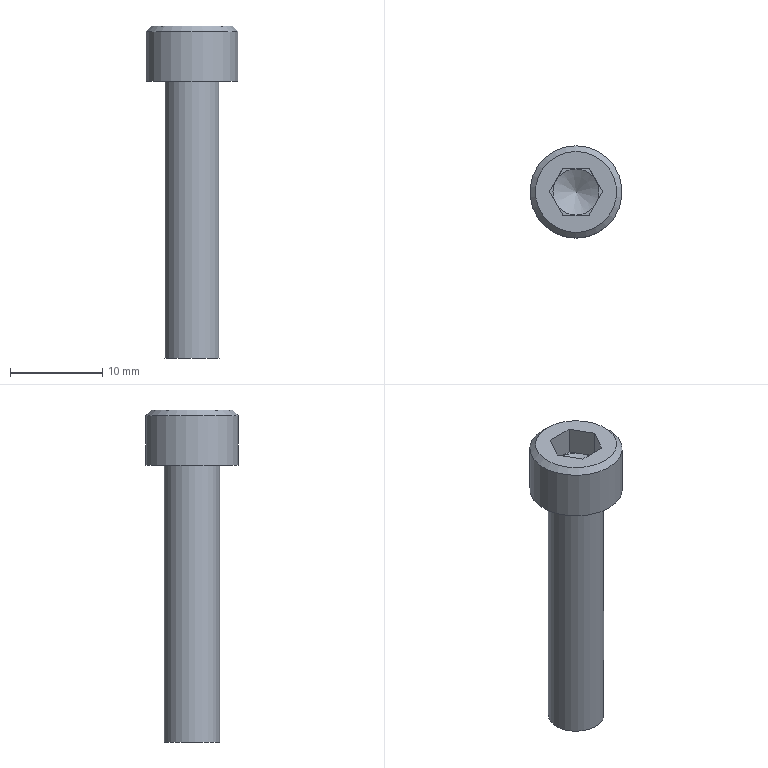Part | NX | features 5003_346_CB6-30 2 | 1 solid | 19 faces | box 10 x 10 x 36 mm | volume 1239 mm3 | plane 15 | cylinder 2 | cone 2 | commonest cylinder face diameters 6 x1 10 x1
STEP:
#1=CARTESIAN_POINT('',(-140.475,32.9,-171.9));
#2=VERTEX_POINT('',#1);
#3=CARTESIAN_POINT('',(-140.475,35.9,-171.9));
#4=DIRECTION('',(0.,0.,1.));
#5=DIRECTION('',(0.,-1.,0.));
#6=AXIS2_PLACEMENT_3D('',#3,#4,#5);
#7=CIRCLE('',#6,3.);
#8=EDGE_CURVE('',#2,#2,#7,.F.);
#9=ORIENTED_EDGE('',*,*,#8,.T.);
#10=EDGE_LOOP('',(#9));
#11=FACE_BOUND('',#10,.T.);
#12=CARTESIAN_POINT('',(-140.475,32.9,-201.9));
#13=VERTEX_POINT('',#12);
#14=CARTESIAN_POINT('',(-140.475,35.9,-201.9));
#15=DIRECTION('',(0.,0.,1.));
#16=DIRECTION('',(0.,-1.,0.));
#17=AXIS2_PLACEMENT_3D('',#14,#15,#16);
#18=CIRCLE('',#17,3.);
#19=EDGE_CURVE('',#13,#13,#18,.T.);
#20=ORIENTED_EDGE('',*,*,#19,.T.);
#21=EDGE_LOOP('',(#20));
#22=FACE_BOUND('',#21,.T.);
#23=CARTESIAN_POINT('',(-140.475,35.9,-165.9));
#24=DIRECTION('',(0.,0.,1.));
#25=DIRECTION('',(0.,-1.,0.));
#26=AXIS2_PLACEMENT_3D('',#23,#24,#25);
#27=CYLINDRICAL_SURFACE('',#26,3.);
#28=ADVANCED_FACE('',(#11,#22),#27,.T.);
#29=ORIENTED_EDGE('',*,*,#8,.F.);
#30=EDGE_LOOP('',(#29));
#31=FACE_BOUND('',#30,.T.);
#32=CARTESIAN_POINT('',(-140.475,30.9,-171.9));
#33=VERTEX_POINT('',#32);
#34=CARTESIAN_POINT('',(-140.475,35.9,-171.9));
#35=DIRECTION('',(0.,0.,1.));
#36=DIRECTION('',(0.,-1.,0.));
#37=AXIS2_PLACEMENT_3D('',#34,#35,#36);
#38=CIRCLE('',#37,5.);
#39=EDGE_CURVE('',#33,#33,#38,.T.);
#40=ORIENTED_EDGE('',*,*,#39,.F.);
#41=EDGE_LOOP('',(#40));
#42=FACE_BOUND('',#41,.T.);
#43=CARTESIAN_POINT('',(-137.475,35.9,-171.9));
#44=DIRECTION('',(0.,0.,1.));
#45=DIRECTION('',(0.,-1.,0.));
#46=AXIS2_PLACEMENT_3D('',#43,#44,#45);
#47=PLANE('',#46);
#48=ADVANCED_FACE('',(#31,#42),#47,.F.);
#49=ORIENTED_EDGE('',*,*,#19,.F.);
#50=EDGE_LOOP('',(#49));
#51=FACE_BOUND('',#50,.T.);
#52=CARTESIAN_POINT('',(-140.475,35.9,-201.9));
#53=DIRECTION('',(0.,0.,1.));
#54=DIRECTION('',(0.,-1.,0.));
#55=AXIS2_PLACEMENT_3D('',#52,#53,#54);
#56=PLANE('',#55);
#57=ADVANCED_FACE('',(#51),#56,.F.);
#58=CARTESIAN_POINT('',(-140.475,30.9,-166.5));
#59=VERTEX_POINT('',#58);
#60=CARTESIAN_POINT('',(-140.475,35.9,-166.5));
#61=DIRECTION('',(0.,0.,1.));
#62=DIRECTION('',(0.,-1.,0.));
#63=AXIS2_PLACEMENT_3D('',#60,#61,#62);
#64=CIRCLE('',#63,5.);
#65=EDGE_CURVE('',#59,#59,#64,.F.);
#66=ORIENTED_EDGE('',*,*,#65,.T.);
#67=EDGE_LOOP('',(#66));
#68=FACE_BOUND('',#67,.T.);
#69=ORIENTED_EDGE('',*,*,#39,.T.);
#70=EDGE_LOOP('',(#69));
#71=FACE_BOUND('',#70,.T.);
#72=CARTESIAN_POINT('',(-140.475,35.9,-165.9));
#73=DIRECTION('',(0.,0.,1.));
#74=DIRECTION('',(0.,-1.,0.));
#75=AXIS2_PLACEMENT_3D('',#72,#73,#74);
#76=CYLINDRICAL_SURFACE('',#75,5.);
#77=ADVANCED_FACE('',(#68,#71),#76,.T.);
#78=ORIENTED_EDGE('',*,*,#65,.F.);
#79=EDGE_LOOP('',(#78));
#80=FACE_BOUND('',#79,.T.);
#81=CARTESIAN_POINT('',(-140.475,40.3,-165.9));
#82=VERTEX_POINT('',#81);
#83=CARTESIAN_POINT('',(-140.475,35.9,-165.9));
#84=DIRECTION('',(0.,0.,-1.));
#85=DIRECTION('',(0.,1.,0.));
#86=AXIS2_PLACEMENT_3D('',#83,#84,#85);
#87=CIRCLE('',#86,4.4);
#88=EDGE_CURVE('',#82,#82,#87,.T.);
#89=ORIENTED_EDGE('',*,*,#88,.T.);
#90=EDGE_LOOP('',(#89));
#91=FACE_BOUND('',#90,.T.);
#92=CARTESIAN_POINT('',(-140.475,35.9,-166.5));
#93=DIRECTION('',(0.,0.,-1.));
#94=DIRECTION('',(0.,1.,0.));
#95=AXIS2_PLACEMENT_3D('',#92,#93,#94);
#96=CONICAL_SURFACE('',#95,5.,0.7854);
#97=ADVANCED_FACE('',(#80,#91),#96,.T.);
#98=CARTESIAN_POINT('',(-141.918,38.4,-165.9));
#99=VERTEX_POINT('',#98);
#100=CARTESIAN_POINT('',(-143.362,35.9,-165.9));
#101=VERTEX_POINT('',#100);
#102=CARTESIAN_POINT('',(-141.918,38.4,-165.9));
#103=DIRECTION('',(-0.5,-0.866,0.));
#104=VECTOR('',#103,1000.);
#105=LINE('',#102,#104);
#106=EDGE_CURVE('',#99,#101,#105,.T.);
#107=ORIENTED_EDGE('',*,*,#106,.F.);
#108=CARTESIAN_POINT('',(-139.032,38.4,-165.9));
#109=VERTEX_POINT('',#108);
#110=CARTESIAN_POINT('',(-135.475,38.4,-165.9));
#111=DIRECTION('',(1.,0.,0.));
#112=VECTOR('',#111,1000.);
#113=LINE('',#110,#112);
#114=EDGE_CURVE('',#109,#99,#113,.F.);
#115=ORIENTED_EDGE('',*,*,#114,.F.);
#116=CARTESIAN_POINT('',(-137.588,35.9,-165.9));
#117=VERTEX_POINT('',#116);
#118=CARTESIAN_POINT('',(-137.588,35.9,-165.9));
#119=DIRECTION('',(-0.5,0.866,0.));
#120=VECTOR('',#119,1000.);
#121=LINE('',#118,#120);
#122=EDGE_CURVE('',#117,#109,#121,.T.);
#123=ORIENTED_EDGE('',*,*,#122,.F.);
#124=CARTESIAN_POINT('',(-139.032,33.4,-165.9));
#125=VERTEX_POINT('',#124);
#126=CARTESIAN_POINT('',(-139.032,33.4,-165.9));
#127=DIRECTION('',(0.5,0.866,0.));
#128=VECTOR('',#127,1000.);
#129=LINE('',#126,#128);
#130=EDGE_CURVE('',#125,#117,#129,.T.);
#131=ORIENTED_EDGE('',*,*,#130,.F.);
#132=CARTESIAN_POINT('',(-141.918,33.4,-165.9));
#133=VERTEX_POINT('',#132);
#134=CARTESIAN_POINT('',(-135.475,33.4,-165.9));
#135=DIRECTION('',(1.,0.,0.));
#136=VECTOR('',#135,1000.);
#137=LINE('',#134,#136);
#138=EDGE_CURVE('',#133,#125,#137,.T.);
#139=ORIENTED_EDGE('',*,*,#138,.F.);
#140=CARTESIAN_POINT('',(-143.362,35.9,-165.9));
#141=DIRECTION('',(0.5,-0.866,0.));
#142=VECTOR('',#141,1000.);
#143=LINE('',#140,#142);
#144=EDGE_CURVE('',#101,#133,#143,.T.);
#145=ORIENTED_EDGE('',*,*,#144,.F.);
#146=EDGE_LOOP('',(#107,#115,#123,#131,#139,#145));
#147=FACE_BOUND('',#146,.T.);
#148=ORIENTED_EDGE('',*,*,#88,.F.);
#149=EDGE_LOOP('',(#148));
#150=FACE_BOUND('',#149,.T.);
#151=CARTESIAN_POINT('',(-135.475,35.9,-165.9));
#152=DIRECTION('',(0.,0.,-1.));
#153=DIRECTION('',(0.,1.,0.));
#154=AXIS2_PLACEMENT_3D('',#151,#152,#153);
#155=PLANE('',#154);
#156=ADVANCED_FACE('',(#147,#150),#155,.F.);
#157=CARTESIAN_POINT('',(-143.362,35.9,-168.9));
#158=VERTEX_POINT('',#157);
#159=CARTESIAN_POINT('',(-143.362,35.9,-168.9));
#160=DIRECTION('',(0.,0.,-1.));
#161=VECTOR('',#160,1000.);
#162=LINE('',#159,#161);
#163=EDGE_CURVE('',#101,#158,#162,.T.);
#164=ORIENTED_EDGE('',*,*,#163,.F.);
#165=ORIENTED_EDGE('',*,*,#144,.T.);
#166=CARTESIAN_POINT('',(-141.918,33.4,-168.9));
#167=VERTEX_POINT('',#166);
#168=CARTESIAN_POINT('',(-141.918,33.4,-168.9));
#169=DIRECTION('',(0.,0.,-1.));
#170=VECTOR('',#169,1000.);
#171=LINE('',#168,#170);
#172=EDGE_CURVE('',#167,#133,#171,.F.);
#173=ORIENTED_EDGE('',*,*,#172,.F.);
#174=CARTESIAN_POINT('',(-142.64,34.65,-168.9));
#175=VERTEX_POINT('',#174);
#176=CARTESIAN_POINT('',(-142.64,34.65,-168.9));
#177=DIRECTION('',(0.5,-0.866,0.));
#178=VECTOR('',#177,1000.);
#179=LINE('',#176,#178);
#180=EDGE_CURVE('',#175,#167,#179,.T.);
#181=ORIENTED_EDGE('',*,*,#180,.F.);
#182=CARTESIAN_POINT('',(-143.362,35.9,-168.9));
#183=DIRECTION('',(-0.5,0.866,0.));
#184=VECTOR('',#183,1000.);
#185=LINE('',#182,#184);
#186=EDGE_CURVE('',#158,#175,#185,.F.);
#187=ORIENTED_EDGE('',*,*,#186,.F.);
#188=EDGE_LOOP('',(#164,#165,#173,#181,#187));
#189=FACE_BOUND('',#188,.T.);
#190=CARTESIAN_POINT('',(-143.362,35.9,-168.9));
#191=DIRECTION('',(-0.866,-0.5,0.));
#192=DIRECTION('',(-0.5,0.866,0.));
#193=AXIS2_PLACEMENT_3D('',#190,#191,#192);
#194=PLANE('',#193);
#195=ADVANCED_FACE('',(#189),#194,.F.);
#196=CARTESIAN_POINT('',(-141.918,38.4,-168.9));
#197=VERTEX_POINT('',#196);
#198=CARTESIAN_POINT('',(-141.918,38.4,-168.9));
#199=DIRECTION('',(0.,0.,-1.));
#200=VECTOR('',#199,1000.);
#201=LINE('',#198,#200);
#202=EDGE_CURVE('',#99,#197,#201,.T.);
#203=ORIENTED_EDGE('',*,*,#202,.F.);
#204=ORIENTED_EDGE('',*,*,#106,.T.);
#205=ORIENTED_EDGE('',*,*,#163,.T.);
#206=CARTESIAN_POINT('',(-142.64,37.15,-168.9));
#207=VERTEX_POINT('',#206);
#208=CARTESIAN_POINT('',(-141.918,38.4,-168.9));
#209=DIRECTION('',(0.5,0.866,0.));
#210=VECTOR('',#209,1000.);
#211=LINE('',#208,#210);
#212=EDGE_CURVE('',#207,#158,#211,.F.);
#213=ORIENTED_EDGE('',*,*,#212,.F.);
#214=CARTESIAN_POINT('',(-141.918,38.4,-168.9));
#215=DIRECTION('',(-0.5,-0.866,0.));
#216=VECTOR('',#215,1000.);
#217=LINE('',#214,#216);
#218=EDGE_CURVE('',#197,#207,#217,.T.);
#219=ORIENTED_EDGE('',*,*,#218,.F.);
#220=EDGE_LOOP('',(#203,#204,#205,#213,#219));
#221=FACE_BOUND('',#220,.T.);
#222=CARTESIAN_POINT('',(-141.918,38.4,-168.9));
#223=DIRECTION('',(-0.866,0.5,0.));
#224=DIRECTION('',(0.5,0.866,0.));
#225=AXIS2_PLACEMENT_3D('',#222,#223,#224);
#226=PLANE('',#225);
#227=ADVANCED_FACE('',(#221),#226,.F.);
#228=CARTESIAN_POINT('',(-139.032,38.4,-168.9));
#229=VERTEX_POINT('',#228);
#230=CARTESIAN_POINT('',(-139.032,38.4,-168.9));
#231=DIRECTION('',(0.,0.,-1.));
#232=VECTOR('',#231,1000.);
#233=LINE('',#230,#232);
#234=EDGE_CURVE('',#109,#229,#233,.T.);
#235=ORIENTED_EDGE('',*,*,#234,.F.);
#236=ORIENTED_EDGE('',*,*,#114,.T.);
#237=ORIENTED_EDGE('',*,*,#202,.T.);
#238=CARTESIAN_POINT('',(-140.475,38.4,-168.9));
#239=VERTEX_POINT('',#238);
#240=CARTESIAN_POINT('',(-140.475,38.4,-168.9));
#241=DIRECTION('',(1.,0.,0.));
#242=VECTOR('',#241,1000.);
#243=LINE('',#240,#242);
#244=EDGE_CURVE('',#239,#197,#243,.F.);
#245=ORIENTED_EDGE('',*,*,#244,.F.);
#246=CARTESIAN_POINT('',(-140.475,38.4,-168.9));
#247=DIRECTION('',(1.,0.,0.));
#248=VECTOR('',#247,1000.);
#249=LINE('',#246,#248);
#250=EDGE_CURVE('',#229,#239,#249,.F.);
#251=ORIENTED_EDGE('',*,*,#250,.F.);
#252=EDGE_LOOP('',(#235,#236,#237,#245,#251));
#253=FACE_BOUND('',#252,.T.);
#254=CARTESIAN_POINT('',(-139.032,38.4,-168.9));
#255=DIRECTION('',(0.,1.,0.));
#256=DIRECTION('',(1.,0.,0.));
#257=AXIS2_PLACEMENT_3D('',#254,#255,#256);
#258=PLANE('',#257);
#259=ADVANCED_FACE('',(#253),#258,.F.);
#260=CARTESIAN_POINT('',(-137.588,35.9,-168.9));
#261=VERTEX_POINT('',#260);
#262=CARTESIAN_POINT('',(-137.588,35.9,-168.9));
#263=DIRECTION('',(0.,0.,-1.));
#264=VECTOR('',#263,1000.);
#265=LINE('',#262,#264);
#266=EDGE_CURVE('',#117,#261,#265,.T.);
#267=ORIENTED_EDGE('',*,*,#266,.F.);
#268=ORIENTED_EDGE('',*,*,#122,.T.);
#269=ORIENTED_EDGE('',*,*,#234,.T.);
#270=CARTESIAN_POINT('',(-138.31,37.15,-168.9));
#271=VERTEX_POINT('',#270);
#272=CARTESIAN_POINT('',(-138.31,37.15,-168.9));
#273=DIRECTION('',(-0.5,0.866,0.));
#274=VECTOR('',#273,1000.);
#275=LINE('',#272,#274);
#276=EDGE_CURVE('',#271,#229,#275,.T.);
#277=ORIENTED_EDGE('',*,*,#276,.F.);
#278=CARTESIAN_POINT('',(-137.588,35.9,-168.9));
#279=DIRECTION('',(0.5,-0.866,0.));
#280=VECTOR('',#279,1000.);
#281=LINE('',#278,#280);
#282=EDGE_CURVE('',#261,#271,#281,.F.);
#283=ORIENTED_EDGE('',*,*,#282,.F.);
#284=EDGE_LOOP('',(#267,#268,#269,#277,#283));
#285=FACE_BOUND('',#284,.T.);
#286=CARTESIAN_POINT('',(-137.588,35.9,-168.9));
#287=DIRECTION('',(0.866,0.5,0.));
#288=DIRECTION('',(0.5,-0.866,0.));
#289=AXIS2_PLACEMENT_3D('',#286,#287,#288);
#290=PLANE('',#289);
#291=ADVANCED_FACE('',(#285),#290,.F.);
#292=CARTESIAN_POINT('',(-139.032,33.4,-168.9));
#293=VERTEX_POINT('',#292);
#294=CARTESIAN_POINT('',(-139.032,33.4,-168.9));
#295=DIRECTION('',(0.,0.,-1.));
#296=VECTOR('',#295,1000.);
#297=LINE('',#294,#296);
#298=EDGE_CURVE('',#125,#293,#297,.T.);
#299=ORIENTED_EDGE('',*,*,#298,.F.);
#300=ORIENTED_EDGE('',*,*,#130,.T.);
#301=ORIENTED_EDGE('',*,*,#266,.T.);
#302=CARTESIAN_POINT('',(-138.31,34.65,-168.9));
#303=VERTEX_POINT('',#302);
#304=CARTESIAN_POINT('',(-139.032,33.4,-168.9));
#305=DIRECTION('',(-0.5,-0.866,0.));
#306=VECTOR('',#305,1000.);
#307=LINE('',#304,#306);
#308=EDGE_CURVE('',#303,#261,#307,.F.);
#309=ORIENTED_EDGE('',*,*,#308,.F.);
#310=CARTESIAN_POINT('',(-139.032,33.4,-168.9));
#311=DIRECTION('',(0.5,0.866,0.));
#312=VECTOR('',#311,1000.);
#313=LINE('',#310,#312);
#314=EDGE_CURVE('',#293,#303,#313,.T.);
#315=ORIENTED_EDGE('',*,*,#314,.F.);
#316=EDGE_LOOP('',(#299,#300,#301,#309,#315));
#317=FACE_BOUND('',#316,.T.);
#318=CARTESIAN_POINT('',(-139.032,33.4,-168.9));
#319=DIRECTION('',(0.866,-0.5,0.));
#320=DIRECTION('',(-0.5,-0.866,0.));
#321=AXIS2_PLACEMENT_3D('',#318,#319,#320);
#322=PLANE('',#321);
#323=ADVANCED_FACE('',(#317),#322,.F.);
#324=ORIENTED_EDGE('',*,*,#172,.T.);
#325=ORIENTED_EDGE('',*,*,#138,.T.);
#326=ORIENTED_EDGE('',*,*,#298,.T.);
#327=CARTESIAN_POINT('',(-140.475,33.4,-168.9));
#328=VERTEX_POINT('',#327);
#329=CARTESIAN_POINT('',(-140.475,33.4,-168.9));
#330=DIRECTION('',(1.,0.,0.));
#331=VECTOR('',#330,1000.);
#332=LINE('',#329,#331);
#333=EDGE_CURVE('',#328,#293,#332,.T.);
#334=ORIENTED_EDGE('',*,*,#333,.F.);
#335=CARTESIAN_POINT('',(-141.918,33.4,-168.9));
#336=DIRECTION('',(1.,0.,0.));
#337=VECTOR('',#336,1000.);
#338=LINE('',#335,#337);
#339=EDGE_CURVE('',#167,#328,#338,.T.);
#340=ORIENTED_EDGE('',*,*,#339,.F.);
#341=EDGE_LOOP('',(#324,#325,#326,#334,#340));
#342=FACE_BOUND('',#341,.T.);
#343=CARTESIAN_POINT('',(-141.918,33.4,-168.9));
#344=DIRECTION('',(0.,-1.,0.));
#345=DIRECTION('',(0.,0.,-1.));
#346=AXIS2_PLACEMENT_3D('',#343,#344,#345);
#347=PLANE('',#346);
#348=ADVANCED_FACE('',(#342),#347,.F.);
#349=CARTESIAN_POINT('',(-140.475,35.9,-168.9));
#350=DIRECTION('',(0.,0.,1.));
#351=DIRECTION('',(-1.,0.,0.));
#352=AXIS2_PLACEMENT_3D('',#349,#350,#351);
#353=CIRCLE('',#352,2.5);
#354=EDGE_CURVE('',#175,#207,#353,.F.);
#355=ORIENTED_EDGE('',*,*,#354,.T.);
#356=ORIENTED_EDGE('',*,*,#212,.T.);
#357=ORIENTED_EDGE('',*,*,#186,.T.);
#358=EDGE_LOOP('',(#355,#356,#357));
#359=FACE_BOUND('',#358,.T.);
#360=CARTESIAN_POINT('',(-140.475,35.9,-168.9));
#361=DIRECTION('',(0.,0.,1.));
#362=DIRECTION('',(0.,-1.,0.));
#363=AXIS2_PLACEMENT_3D('',#360,#361,#362);
#364=PLANE('',#363);
#365=ADVANCED_FACE('',(#359),#364,.T.);
#366=ORIENTED_EDGE('',*,*,#282,.T.);
#367=CARTESIAN_POINT('',(-140.475,35.9,-168.9));
#368=DIRECTION('',(0.,0.,1.));
#369=DIRECTION('',(-1.,0.,0.));
#370=AXIS2_PLACEMENT_3D('',#367,#368,#369);
#371=CIRCLE('',#370,2.5);
#372=EDGE_CURVE('',#271,#303,#371,.F.);
#373=ORIENTED_EDGE('',*,*,#372,.T.);
#374=ORIENTED_EDGE('',*,*,#308,.T.);
#375=EDGE_LOOP('',(#366,#373,#374));
#376=FACE_BOUND('',#375,.T.);
#377=CARTESIAN_POINT('',(-140.475,35.9,-168.9));
#378=DIRECTION('',(0.,0.,1.));
#379=DIRECTION('',(0.,-1.,0.));
#380=AXIS2_PLACEMENT_3D('',#377,#378,#379);
#381=PLANE('',#380);
#382=ADVANCED_FACE('',(#376),#381,.T.);
#383=ORIENTED_EDGE('',*,*,#339,.T.);
#384=CARTESIAN_POINT('',(-140.475,35.9,-168.9));
#385=DIRECTION('',(0.,0.,1.));
#386=DIRECTION('',(-1.,0.,0.));
#387=AXIS2_PLACEMENT_3D('',#384,#385,#386);
#388=CIRCLE('',#387,2.5);
#389=EDGE_CURVE('',#328,#175,#388,.F.);
#390=ORIENTED_EDGE('',*,*,#389,.T.);
#391=ORIENTED_EDGE('',*,*,#180,.T.);
#392=EDGE_LOOP('',(#383,#390,#391));
#393=FACE_BOUND('',#392,.T.);
#394=CARTESIAN_POINT('',(-140.475,35.9,-168.9));
#395=DIRECTION('',(0.,0.,1.));
#396=DIRECTION('',(0.,-1.,0.));
#397=AXIS2_PLACEMENT_3D('',#394,#395,#396);
#398=PLANE('',#397);
#399=ADVANCED_FACE('',(#393),#398,.T.);
#400=CARTESIAN_POINT('',(-140.475,35.9,-170.402));
#401=VERTEX_POINT('',#400);
#402=VERTEX_LOOP('',#401);
#403=FACE_BOUND('',#402,.T.);
#404=CARTESIAN_POINT('',(-140.475,35.9,-168.9));
#405=DIRECTION('',(0.,0.,1.));
#406=DIRECTION('',(-1.,0.,0.));
#407=AXIS2_PLACEMENT_3D('',#404,#405,#406);
#408=CIRCLE('',#407,2.5);
#409=EDGE_CURVE('',#207,#239,#408,.F.);
#410=ORIENTED_EDGE('',*,*,#409,.F.);
#411=ORIENTED_EDGE('',*,*,#354,.F.);
#412=ORIENTED_EDGE('',*,*,#389,.F.);
#413=CARTESIAN_POINT('',(-140.475,35.9,-168.9));
#414=DIRECTION('',(0.,0.,1.));
#415=DIRECTION('',(-1.,0.,0.));
#416=AXIS2_PLACEMENT_3D('',#413,#414,#415);
#417=CIRCLE('',#416,2.5);
#418=EDGE_CURVE('',#303,#328,#417,.F.);
#419=ORIENTED_EDGE('',*,*,#418,.F.);
#420=ORIENTED_EDGE('',*,*,#372,.F.);
#421=CARTESIAN_POINT('',(-140.475,35.9,-168.9));
#422=DIRECTION('',(0.,0.,1.));
#423=DIRECTION('',(-1.,0.,0.));
#424=AXIS2_PLACEMENT_3D('',#421,#422,#423);
#425=CIRCLE('',#424,2.5);
#426=EDGE_CURVE('',#239,#271,#425,.F.);
#427=ORIENTED_EDGE('',*,*,#426,.F.);
#428=EDGE_LOOP('',(#410,#411,#412,#419,#420,#427));
#429=FACE_BOUND('',#428,.T.);
#430=CARTESIAN_POINT('',(-140.475,35.9,-168.9));
#431=DIRECTION('',(0.,0.,1.));
#432=DIRECTION('',(-1.,0.,0.));
#433=AXIS2_PLACEMENT_3D('',#430,#431,#432);
#434=CONICAL_SURFACE('',#433,2.5,1.03);
#435=ADVANCED_FACE('',(#403,#429),#434,.F.);
#436=ORIENTED_EDGE('',*,*,#314,.T.);
#437=ORIENTED_EDGE('',*,*,#418,.T.);
#438=ORIENTED_EDGE('',*,*,#333,.T.);
#439=EDGE_LOOP('',(#436,#437,#438));
#440=FACE_BOUND('',#439,.T.);
#441=CARTESIAN_POINT('',(-140.475,35.9,-168.9));
#442=DIRECTION('',(0.,0.,1.));
#443=DIRECTION('',(0.,-1.,0.));
#444=AXIS2_PLACEMENT_3D('',#441,#442,#443);
#445=PLANE('',#444);
#446=ADVANCED_FACE('',(#440),#445,.T.);
#447=ORIENTED_EDGE('',*,*,#250,.T.);
#448=ORIENTED_EDGE('',*,*,#426,.T.);
#449=ORIENTED_EDGE('',*,*,#276,.T.);
#450=EDGE_LOOP('',(#447,#448,#449));
#451=FACE_BOUND('',#450,.T.);
#452=CARTESIAN_POINT('',(-140.475,35.9,-168.9));
#453=DIRECTION('',(0.,0.,1.));
#454=DIRECTION('',(0.,-1.,0.));
#455=AXIS2_PLACEMENT_3D('',#452,#453,#454);
#456=PLANE('',#455);
#457=ADVANCED_FACE('',(#451),#456,.T.);
#458=ORIENTED_EDGE('',*,*,#218,.T.);
#459=ORIENTED_EDGE('',*,*,#409,.T.);
#460=ORIENTED_EDGE('',*,*,#244,.T.);
#461=EDGE_LOOP('',(#458,#459,#460));
#462=FACE_BOUND('',#461,.T.);
#463=CARTESIAN_POINT('',(-140.475,35.9,-168.9));
#464=DIRECTION('',(0.,0.,1.));
#465=DIRECTION('',(0.,-1.,0.));
#466=AXIS2_PLACEMENT_3D('',#463,#464,#465);
#467=PLANE('',#466);
#468=ADVANCED_FACE('',(#462),#467,.T.);
#469=CLOSED_SHELL('',(#28,#48,#57,#77,#97,#156,#195,#227,#259,#291,#323,#348,#365,#382,#399,#435,#446,#457,#468));
#470=MANIFOLD_SOLID_BREP('',#469);
#471=(LENGTH_UNIT()NAMED_UNIT(*)SI_UNIT(.MILLI.,.METRE.));
#472=UNCERTAINTY_MEASURE_WITH_UNIT(LENGTH_MEASURE(0.00001),#471,'','');
#473=(NAMED_UNIT(*)PLANE_ANGLE_UNIT()SI_UNIT($,.RADIAN.));
#474=(NAMED_UNIT(*)SI_UNIT($,.STERADIAN.)SOLID_ANGLE_UNIT());
#475=(GEOMETRIC_REPRESENTATION_CONTEXT(3)GLOBAL_UNCERTAINTY_ASSIGNED_CONTEXT((#472))GLOBAL_UNIT_ASSIGNED_CONTEXT((#471,#473,#474))REPRESENTATION_CONTEXT('',''));
#476=ADVANCED_BREP_SHAPE_REPRESENTATION('',(#470),#475);